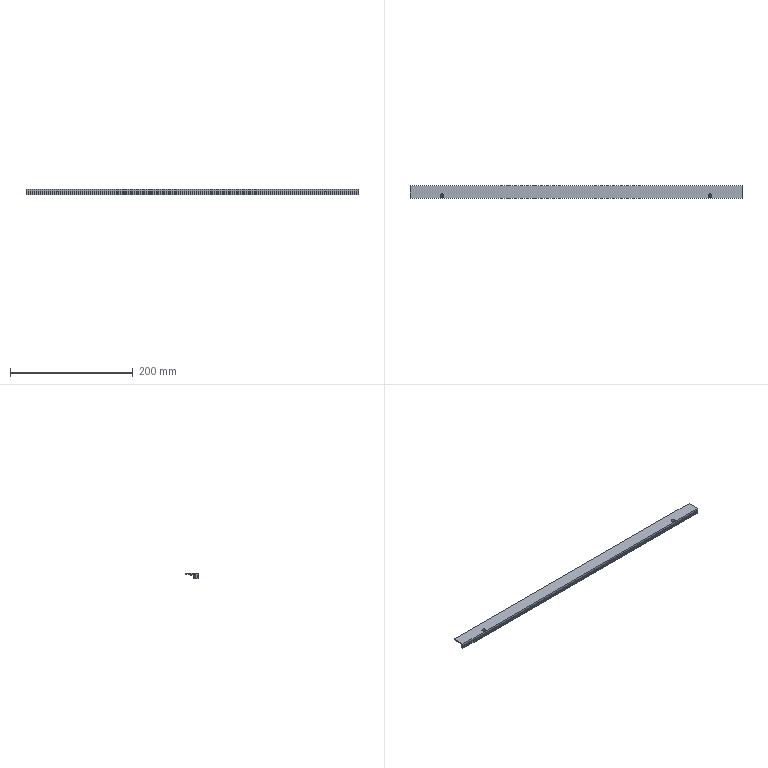Part | SolidWorks | features BaseBody 1 | 1 solid | 40 faces | box 540 x 20 x 9 mm | volume 48974 mm3 | plane 26 | cylinder 12 | cone 2 | commonest cylinder face diameters 6 x6 3.3 x4 2.076 x2
STEP:
#1=CARTESIAN_POINT('',(-215.,-187.,12.));
#2=VERTEX_POINT('',#1);
#3=CARTESIAN_POINT('',(-221.,-187.,12.));
#4=VERTEX_POINT('',#3);
#5=CARTESIAN_POINT('',(-218.,-187.,12.));
#6=DIRECTION('',(0.,0.,-1.));
#7=DIRECTION('',(-1.,0.,0.));
#8=AXIS2_PLACEMENT_3D('',#5,#6,#7);
#9=CIRCLE('',#8,3.);
#10=EDGE_CURVE('',#2,#4,#9,.T.);
#11=ORIENTED_EDGE('',*,*,#10,.F.);
#12=CARTESIAN_POINT('',(-215.,-187.,8.8));
#13=VERTEX_POINT('',#12);
#14=CARTESIAN_POINT('',(-215.,-187.,10.4));
#15=DIRECTION('',(0.,0.,-1.));
#16=VECTOR('',#15,1000.);
#17=LINE('',#14,#16);
#18=EDGE_CURVE('',#2,#13,#17,.T.);
#19=ORIENTED_EDGE('',*,*,#18,.T.);
#20=CARTESIAN_POINT('',(-221.,-187.,8.8));
#21=VERTEX_POINT('',#20);
#22=CARTESIAN_POINT('',(-218.,-187.,8.8));
#23=DIRECTION('',(0.,0.,1.));
#24=DIRECTION('',(-1.,0.,0.));
#25=AXIS2_PLACEMENT_3D('',#22,#23,#24);
#26=CIRCLE('',#25,3.);
#27=EDGE_CURVE('',#21,#13,#26,.T.);
#28=ORIENTED_EDGE('',*,*,#27,.F.);
#29=CARTESIAN_POINT('',(-221.,-187.,10.4));
#30=DIRECTION('',(0.,0.,-1.));
#31=VECTOR('',#30,1000.);
#32=LINE('',#29,#31);
#33=EDGE_CURVE('',#4,#21,#32,.T.);
#34=ORIENTED_EDGE('',*,*,#33,.F.);
#35=EDGE_LOOP('',(#11,#19,#28,#34));
#36=FACE_OUTER_BOUND('',#35,.T.);
#37=CARTESIAN_POINT('',(-218.,-187.,10.4));
#38=DIRECTION('',(0.,0.,-1.));
#39=DIRECTION('',(-1.,0.,0.));
#40=AXIS2_PLACEMENT_3D('',#37,#38,#39);
#41=CYLINDRICAL_SURFACE('',#40,3.);
#42=ADVANCED_FACE('',(#36),#41,.F.);
#43=CARTESIAN_POINT('',(221.,-187.,12.));
#44=VERTEX_POINT('',#43);
#45=CARTESIAN_POINT('',(215.,-187.,12.));
#46=VERTEX_POINT('',#45);
#47=CARTESIAN_POINT('',(218.,-187.,12.));
#48=DIRECTION('',(0.,0.,-1.));
#49=DIRECTION('',(-1.,0.,0.));
#50=AXIS2_PLACEMENT_3D('',#47,#48,#49);
#51=CIRCLE('',#50,3.);
#52=EDGE_CURVE('',#44,#46,#51,.T.);
#53=ORIENTED_EDGE('',*,*,#52,.F.);
#54=CARTESIAN_POINT('',(221.,-187.,8.8));
#55=VERTEX_POINT('',#54);
#56=CARTESIAN_POINT('',(221.,-187.,10.4));
#57=DIRECTION('',(0.,0.,-1.));
#58=VECTOR('',#57,1000.);
#59=LINE('',#56,#58);
#60=EDGE_CURVE('',#44,#55,#59,.T.);
#61=ORIENTED_EDGE('',*,*,#60,.T.);
#62=CARTESIAN_POINT('',(215.,-187.,8.8));
#63=VERTEX_POINT('',#62);
#64=CARTESIAN_POINT('',(218.,-187.,8.8));
#65=DIRECTION('',(0.,0.,1.));
#66=DIRECTION('',(-1.,0.,0.));
#67=AXIS2_PLACEMENT_3D('',#64,#65,#66);
#68=CIRCLE('',#67,3.);
#69=EDGE_CURVE('',#63,#55,#68,.T.);
#70=ORIENTED_EDGE('',*,*,#69,.F.);
#71=CARTESIAN_POINT('',(215.,-187.,10.4));
#72=DIRECTION('',(0.,0.,-1.));
#73=VECTOR('',#72,1000.);
#74=LINE('',#71,#73);
#75=EDGE_CURVE('',#46,#63,#74,.T.);
#76=ORIENTED_EDGE('',*,*,#75,.F.);
#77=EDGE_LOOP('',(#53,#61,#70,#76));
#78=FACE_OUTER_BOUND('',#77,.T.);
#79=CARTESIAN_POINT('',(218.,-187.,10.4));
#80=DIRECTION('',(0.,0.,-1.));
#81=DIRECTION('',(-1.,0.,0.));
#82=AXIS2_PLACEMENT_3D('',#79,#80,#81);
#83=CYLINDRICAL_SURFACE('',#82,3.);
#84=ADVANCED_FACE('',(#78),#83,.F.);
#85=CARTESIAN_POINT('',(-219.65,-187.,8.8));
#86=VERTEX_POINT('',#85);
#87=CARTESIAN_POINT('',(-216.35,-187.,8.8));
#88=VERTEX_POINT('',#87);
#89=CARTESIAN_POINT('',(-218.,-187.,8.8));
#90=DIRECTION('',(0.,0.,1.));
#91=DIRECTION('',(-1.,0.,0.));
#92=AXIS2_PLACEMENT_3D('',#89,#90,#91);
#93=CIRCLE('',#92,1.65);
#94=EDGE_CURVE('',#86,#88,#93,.T.);
#95=ORIENTED_EDGE('',*,*,#94,.T.);
#96=CARTESIAN_POINT('',(-216.35,-187.,3.));
#97=VERTEX_POINT('',#96);
#98=CARTESIAN_POINT('',(-216.35,-187.,7.));
#99=DIRECTION('',(0.,0.,-1.));
#100=VECTOR('',#99,1000.);
#101=LINE('',#98,#100);
#102=EDGE_CURVE('',#88,#97,#101,.T.);
#103=ORIENTED_EDGE('',*,*,#102,.T.);
#104=CARTESIAN_POINT('',(-219.65,-187.,3.));
#105=VERTEX_POINT('',#104);
#106=CARTESIAN_POINT('',(-218.,-187.,3.));
#107=DIRECTION('',(0.,0.,1.));
#108=DIRECTION('',(-1.,0.,0.));
#109=AXIS2_PLACEMENT_3D('',#106,#107,#108);
#110=CIRCLE('',#109,1.65);
#111=EDGE_CURVE('',#105,#97,#110,.T.);
#112=ORIENTED_EDGE('',*,*,#111,.F.);
#113=CARTESIAN_POINT('',(-219.65,-187.,7.));
#114=DIRECTION('',(0.,0.,-1.));
#115=VECTOR('',#114,1000.);
#116=LINE('',#113,#115);
#117=EDGE_CURVE('',#86,#105,#116,.T.);
#118=ORIENTED_EDGE('',*,*,#117,.F.);
#119=EDGE_LOOP('',(#95,#103,#112,#118));
#120=FACE_OUTER_BOUND('',#119,.T.);
#121=CARTESIAN_POINT('',(-218.,-187.,7.));
#122=DIRECTION('',(0.,0.,-1.));
#123=DIRECTION('',(-1.,0.,0.));
#124=AXIS2_PLACEMENT_3D('',#121,#122,#123);
#125=CYLINDRICAL_SURFACE('',#124,1.65);
#126=ADVANCED_FACE('',(#120),#125,.F.);
#127=CARTESIAN_POINT('',(216.35,-187.,8.8));
#128=VERTEX_POINT('',#127);
#129=CARTESIAN_POINT('',(219.65,-187.,8.8));
#130=VERTEX_POINT('',#129);
#131=CARTESIAN_POINT('',(218.,-187.,8.8));
#132=DIRECTION('',(0.,0.,1.));
#133=DIRECTION('',(-1.,0.,0.));
#134=AXIS2_PLACEMENT_3D('',#131,#132,#133);
#135=CIRCLE('',#134,1.65);
#136=EDGE_CURVE('',#128,#130,#135,.T.);
#137=ORIENTED_EDGE('',*,*,#136,.T.);
#138=CARTESIAN_POINT('',(219.65,-187.,3.));
#139=VERTEX_POINT('',#138);
#140=CARTESIAN_POINT('',(219.65,-187.,7.));
#141=DIRECTION('',(0.,0.,-1.));
#142=VECTOR('',#141,1000.);
#143=LINE('',#140,#142);
#144=EDGE_CURVE('',#130,#139,#143,.T.);
#145=ORIENTED_EDGE('',*,*,#144,.T.);
#146=CARTESIAN_POINT('',(216.35,-187.,3.));
#147=VERTEX_POINT('',#146);
#148=CARTESIAN_POINT('',(218.,-187.,3.));
#149=DIRECTION('',(0.,0.,1.));
#150=DIRECTION('',(-1.,0.,0.));
#151=AXIS2_PLACEMENT_3D('',#148,#149,#150);
#152=CIRCLE('',#151,1.65);
#153=EDGE_CURVE('',#147,#139,#152,.T.);
#154=ORIENTED_EDGE('',*,*,#153,.F.);
#155=CARTESIAN_POINT('',(216.35,-187.,7.));
#156=DIRECTION('',(0.,0.,-1.));
#157=VECTOR('',#156,1000.);
#158=LINE('',#155,#157);
#159=EDGE_CURVE('',#128,#147,#158,.T.);
#160=ORIENTED_EDGE('',*,*,#159,.F.);
#161=EDGE_LOOP('',(#137,#145,#154,#160));
#162=FACE_OUTER_BOUND('',#161,.T.);
#163=CARTESIAN_POINT('',(218.,-187.,7.));
#164=DIRECTION('',(0.,0.,-1.));
#165=DIRECTION('',(-1.,0.,0.));
#166=AXIS2_PLACEMENT_3D('',#163,#164,#165);
#167=CYLINDRICAL_SURFACE('',#166,1.65);
#168=ADVANCED_FACE('',(#162),#167,.F.);
#169=CARTESIAN_POINT('',(-254.,-184.,6.223));
#170=VERTEX_POINT('',#169);
#171=CARTESIAN_POINT('',(-254.798,-186.038,6.5));
#172=VERTEX_POINT('',#171);
#173=CARTESIAN_POINT('',(-254.,-184.,6.223));
#174=CARTESIAN_POINT('',(-254.,-184.035,6.096));
#175=CARTESIAN_POINT('',(-254.,-184.093,5.978));
#176=CARTESIAN_POINT('',(-254.009,-184.251,5.77));
#177=CARTESIAN_POINT('',(-254.018,-184.349,5.681));
#178=CARTESIAN_POINT('',(-254.052,-184.569,5.547));
#179=CARTESIAN_POINT('',(-254.078,-184.692,5.501));
#180=CARTESIAN_POINT('',(-254.148,-184.938,5.457));
#181=CARTESIAN_POINT('',(-254.192,-185.064,5.457));
#182=CARTESIAN_POINT('',(-254.343,-185.417,5.52));
#183=CARTESIAN_POINT('',(-254.473,-185.628,5.641));
#184=CARTESIAN_POINT('',(-254.642,-185.858,5.904));
#185=CARTESIAN_POINT('',(-254.696,-185.922,6.008));
#186=CARTESIAN_POINT('',(-254.774,-186.012,6.239));
#187=CARTESIAN_POINT('',(-254.798,-186.038,6.368));
#188=CARTESIAN_POINT('',(-254.798,-186.038,6.5));
#189=B_SPLINE_CURVE_WITH_KNOTS('',3,(#173,#174,#175,#176,#177,#178,#179,#180,#181,#182,#183,#184,#185,#186,#187,#188),.UNSPECIFIED.,.F.,.F.,(4,2,2,2,2,2,2,4),(0.,0.000389,0.000778,0.001167,0.001556,0.002334,0.002723,0.003112),.UNSPECIFIED.);
#190=EDGE_CURVE('',#170,#172,#189,.T.);
#191=ORIENTED_EDGE('',*,*,#190,.T.);
#192=CARTESIAN_POINT('',(-219.34,-186.038,6.5));
#193=VERTEX_POINT('',#192);
#194=CARTESIAN_POINT('',(-150.,-186.038,6.5));
#195=DIRECTION('',(1.,0.,0.));
#196=VECTOR('',#195,1000.);
#197=LINE('',#194,#196);
#198=EDGE_CURVE('',#172,#193,#197,.T.);
#199=ORIENTED_EDGE('',*,*,#198,.T.);
#200=CARTESIAN_POINT('',(-216.66,-186.038,6.5));
#201=VERTEX_POINT('',#200);
#202=CARTESIAN_POINT('',(-219.34,-186.038,6.5));
#203=CARTESIAN_POINT('',(-219.34,-186.038,6.328));
#204=CARTESIAN_POINT('',(-219.31,-185.991,6.154));
#205=CARTESIAN_POINT('',(-219.18,-185.842,5.873));
#206=CARTESIAN_POINT('',(-219.077,-185.741,5.764));
#207=CARTESIAN_POINT('',(-218.821,-185.56,5.619));
#208=CARTESIAN_POINT('',(-218.668,-185.482,5.579));
#209=CARTESIAN_POINT('',(-218.345,-185.378,5.532));
#210=CARTESIAN_POINT('',(-218.172,-185.35,5.523));
#211=CARTESIAN_POINT('',(-217.828,-185.35,5.523));
#212=CARTESIAN_POINT('',(-217.656,-185.377,5.532));
#213=CARTESIAN_POINT('',(-217.413,-185.456,5.567));
#214=CARTESIAN_POINT('',(-217.333,-185.488,5.583));
#215=CARTESIAN_POINT('',(-217.185,-185.563,5.627));
#216=CARTESIAN_POINT('',(-217.115,-185.605,5.655));
#217=CARTESIAN_POINT('',(-216.986,-185.696,5.728));
#218=CARTESIAN_POINT('',(-216.929,-185.743,5.772));
#219=CARTESIAN_POINT('',(-216.83,-185.835,5.88));
#220=CARTESIAN_POINT('',(-216.788,-185.879,5.943));
#221=CARTESIAN_POINT('',(-216.691,-185.991,6.153));
#222=CARTESIAN_POINT('',(-216.66,-186.038,6.326));
#223=CARTESIAN_POINT('',(-216.66,-186.038,6.5));
#224=B_SPLINE_CURVE_WITH_KNOTS('',3,(#202,#203,#204,#205,#206,#207,#208,#209,#210,#211,#212,#213,#214,#215,#216,#217,#218,#219,#220,#221,#222,#223),.UNSPECIFIED.,.F.,.F.,(4,2,2,2,2,2,2,2,2,2,4),(0.004127,0.004642,0.005157,0.005672,0.006187,0.006702,0.00696,0.007217,0.007475,0.007733,0.008248),.UNSPECIFIED.);
#225=EDGE_CURVE('',#193,#201,#224,.T.);
#226=ORIENTED_EDGE('',*,*,#225,.T.);
#227=CARTESIAN_POINT('',(-30.,-186.038,6.5));
#228=VERTEX_POINT('',#227);
#229=CARTESIAN_POINT('',(-150.,-186.038,6.5));
#230=DIRECTION('',(1.,0.,0.));
#231=VECTOR('',#230,1000.);
#232=LINE('',#229,#231);
#233=EDGE_CURVE('',#201,#228,#232,.T.);
#234=ORIENTED_EDGE('',*,*,#233,.T.);
#235=CARTESIAN_POINT('',(-30.,-185.,5.462));
#236=VERTEX_POINT('',#235);
#237=CARTESIAN_POINT('',(-30.,-185.,6.5));
#238=DIRECTION('',(-1.,0.,0.));
#239=DIRECTION('',(0.,1.,0.));
#240=AXIS2_PLACEMENT_3D('',#237,#238,#239);
#241=CIRCLE('',#240,1.038);
#242=EDGE_CURVE('',#236,#228,#241,.T.);
#243=ORIENTED_EDGE('',*,*,#242,.F.);
#244=CARTESIAN_POINT('',(-30.,-183.962,6.5));
#245=VERTEX_POINT('',#244);
#246=CARTESIAN_POINT('',(-30.,-185.,6.5));
#247=DIRECTION('',(-1.,0.,0.));
#248=DIRECTION('',(0.,1.,0.));
#249=AXIS2_PLACEMENT_3D('',#246,#247,#248);
#250=CIRCLE('',#249,1.038);
#251=EDGE_CURVE('',#245,#236,#250,.T.);
#252=ORIENTED_EDGE('',*,*,#251,.F.);
#253=CARTESIAN_POINT('',(-254.,-183.962,6.5));
#254=VERTEX_POINT('',#253);
#255=CARTESIAN_POINT('',(-150.,-183.962,6.5));
#256=DIRECTION('',(1.,0.,0.));
#257=VECTOR('',#256,1000.);
#258=LINE('',#255,#257);
#259=EDGE_CURVE('',#254,#245,#258,.T.);
#260=ORIENTED_EDGE('',*,*,#259,.F.);
#261=CARTESIAN_POINT('',(-254.,-185.,6.5));
#262=DIRECTION('',(-1.,0.,0.));
#263=DIRECTION('',(0.,1.,0.));
#264=AXIS2_PLACEMENT_3D('',#261,#262,#263);
#265=CIRCLE('',#264,1.038);
#266=EDGE_CURVE('',#254,#170,#265,.T.);
#267=ORIENTED_EDGE('',*,*,#266,.T.);
#268=EDGE_LOOP('',(#191,#199,#226,#234,#243,#252,#260,#267));
#269=FACE_OUTER_BOUND('',#268,.T.);
#270=CARTESIAN_POINT('',(-150.,-185.,6.5));
#271=DIRECTION('',(1.,0.,0.));
#272=DIRECTION('',(0.,1.,0.));
#273=AXIS2_PLACEMENT_3D('',#270,#271,#272);
#274=CYLINDRICAL_SURFACE('',#273,1.038);
#275=ADVANCED_FACE('',(#269),#274,.F.);
#276=CARTESIAN_POINT('',(-29.376,-185.,6.5));
#277=VERTEX_POINT('',#276);
#278=CARTESIAN_POINT('',(-30.,-185.,7.538));
#279=VERTEX_POINT('',#278);
#280=CARTESIAN_POINT('',(-30.,-185.,7.538));
#281=DIRECTION('',(-0.515,0.,0.8572));
#282=VECTOR('',#281,1000.);
#283=LINE('',#280,#282);
#284=EDGE_CURVE('',#277,#279,#283,.T.);
#285=ORIENTED_EDGE('',*,*,#284,.F.);
#286=CARTESIAN_POINT('',(-30.,-185.,5.462));
#287=DIRECTION('',(-0.515,0.,-0.8572));
#288=VECTOR('',#287,1000.);
#289=LINE('',#286,#288);
#290=EDGE_CURVE('',#277,#236,#289,.T.);
#291=ORIENTED_EDGE('',*,*,#290,.T.);
#292=ORIENTED_EDGE('',*,*,#242,.T.);
#293=CARTESIAN_POINT('',(-30.,-185.,6.5));
#294=DIRECTION('',(-1.,0.,0.));
#295=DIRECTION('',(0.,1.,0.));
#296=AXIS2_PLACEMENT_3D('',#293,#294,#295);
#297=CIRCLE('',#296,1.038);
#298=EDGE_CURVE('',#228,#279,#297,.T.);
#299=ORIENTED_EDGE('',*,*,#298,.T.);
#300=EDGE_LOOP('',(#285,#291,#292,#299));
#301=FACE_OUTER_BOUND('',#300,.T.);
#302=CARTESIAN_POINT('',(-30.,-185.,6.5));
#303=DIRECTION('',(-1.,0.,0.));
#304=DIRECTION('',(0.,0.,1.));
#305=AXIS2_PLACEMENT_3D('',#302,#303,#304);
#306=CONICAL_SURFACE('',#305,1.038,1.03);
#307=ADVANCED_FACE('',(#301),#306,.F.);
#308=CARTESIAN_POINT('',(-218.,-187.,12.));
#309=DIRECTION('',(0.,0.,-1.));
#310=DIRECTION('',(-1.,0.,0.));
#311=AXIS2_PLACEMENT_3D('',#308,#309,#310);
#312=CIRCLE('',#311,3.);
#313=EDGE_CURVE('',#4,#2,#312,.T.);
#314=ORIENTED_EDGE('',*,*,#313,.T.);
#315=ORIENTED_EDGE('',*,*,#10,.T.);
#316=EDGE_LOOP('',(#314,#315));
#317=FACE_BOUND('',#316,.T.);
#318=CARTESIAN_POINT('',(218.,-187.,12.));
#319=DIRECTION('',(0.,0.,-1.));
#320=DIRECTION('',(-1.,0.,0.));
#321=AXIS2_PLACEMENT_3D('',#318,#319,#320);
#322=CIRCLE('',#321,3.);
#323=EDGE_CURVE('',#46,#44,#322,.T.);
#324=ORIENTED_EDGE('',*,*,#323,.T.);
#325=ORIENTED_EDGE('',*,*,#52,.T.);
#326=EDGE_LOOP('',(#324,#325));
#327=FACE_BOUND('',#326,.T.);
#328=CARTESIAN_POINT('',(-270.,-171.,12.));
#329=VERTEX_POINT('',#328);
#330=CARTESIAN_POINT('',(-270.,-191.,12.));
#331=VERTEX_POINT('',#330);
#332=CARTESIAN_POINT('',(-270.,-171.,12.));
#333=DIRECTION('',(0.,-1.,0.));
#334=VECTOR('',#333,1000.);
#335=LINE('',#332,#334);
#336=EDGE_CURVE('',#329,#331,#335,.T.);
#337=ORIENTED_EDGE('',*,*,#336,.T.);
#338=CARTESIAN_POINT('',(270.,-191.,12.));
#339=VERTEX_POINT('',#338);
#340=CARTESIAN_POINT('',(-270.,-191.,12.));
#341=DIRECTION('',(1.,0.,0.));
#342=VECTOR('',#341,1000.);
#343=LINE('',#340,#342);
#344=EDGE_CURVE('',#331,#339,#343,.T.);
#345=ORIENTED_EDGE('',*,*,#344,.T.);
#346=CARTESIAN_POINT('',(270.,-171.,12.));
#347=VERTEX_POINT('',#346);
#348=CARTESIAN_POINT('',(270.,-171.,12.));
#349=DIRECTION('',(0.,1.,0.));
#350=VECTOR('',#349,1000.);
#351=LINE('',#348,#350);
#352=EDGE_CURVE('',#339,#347,#351,.T.);
#353=ORIENTED_EDGE('',*,*,#352,.T.);
#354=CARTESIAN_POINT('',(-270.,-171.,12.));
#355=DIRECTION('',(-1.,0.,0.));
#356=VECTOR('',#355,1000.);
#357=LINE('',#354,#356);
#358=EDGE_CURVE('',#347,#329,#357,.T.);
#359=ORIENTED_EDGE('',*,*,#358,.T.);
#360=EDGE_LOOP('',(#337,#345,#353,#359));
#361=FACE_OUTER_BOUND('',#360,.T.);
#362=CARTESIAN_POINT('',(-270.,-171.,12.));
#363=DIRECTION('',(0.,0.,1.));
#364=DIRECTION('',(1.,0.,0.));
#365=AXIS2_PLACEMENT_3D('',#362,#363,#364);
#366=PLANE('',#365);
#367=ADVANCED_FACE('',(#317,#327,#361),#366,.T.);
#368=ORIENTED_EDGE('',*,*,#18,.F.);
#369=ORIENTED_EDGE('',*,*,#313,.F.);
#370=ORIENTED_EDGE('',*,*,#33,.T.);
#371=CARTESIAN_POINT('',(-218.,-187.,8.8));
#372=DIRECTION('',(0.,0.,1.));
#373=DIRECTION('',(-1.,0.,0.));
#374=AXIS2_PLACEMENT_3D('',#371,#372,#373);
#375=CIRCLE('',#374,3.);
#376=EDGE_CURVE('',#13,#21,#375,.T.);
#377=ORIENTED_EDGE('',*,*,#376,.F.);
#378=EDGE_LOOP('',(#368,#369,#370,#377));
#379=FACE_OUTER_BOUND('',#378,.T.);
#380=CARTESIAN_POINT('',(-218.,-187.,10.4));
#381=DIRECTION('',(0.,0.,-1.));
#382=DIRECTION('',(-1.,0.,0.));
#383=AXIS2_PLACEMENT_3D('',#380,#381,#382);
#384=CYLINDRICAL_SURFACE('',#383,3.);
#385=ADVANCED_FACE('',(#379),#384,.F.);
#386=ORIENTED_EDGE('',*,*,#60,.F.);
#387=ORIENTED_EDGE('',*,*,#323,.F.);
#388=ORIENTED_EDGE('',*,*,#75,.T.);
#389=CARTESIAN_POINT('',(218.,-187.,8.8));
#390=DIRECTION('',(0.,0.,1.));
#391=DIRECTION('',(-1.,0.,0.));
#392=AXIS2_PLACEMENT_3D('',#389,#390,#391);
#393=CIRCLE('',#392,3.);
#394=EDGE_CURVE('',#55,#63,#393,.T.);
#395=ORIENTED_EDGE('',*,*,#394,.F.);
#396=EDGE_LOOP('',(#386,#387,#388,#395));
#397=FACE_OUTER_BOUND('',#396,.T.);
#398=CARTESIAN_POINT('',(218.,-187.,10.4));
#399=DIRECTION('',(0.,0.,-1.));
#400=DIRECTION('',(-1.,0.,0.));
#401=AXIS2_PLACEMENT_3D('',#398,#399,#400);
#402=CYLINDRICAL_SURFACE('',#401,3.);
#403=ADVANCED_FACE('',(#397),#402,.F.);
#404=ORIENTED_EDGE('',*,*,#344,.F.);
#405=CARTESIAN_POINT('',(-270.,-191.,8.5));
#406=VERTEX_POINT('',#405);
#407=CARTESIAN_POINT('',(-270.,-191.,12.));
#408=DIRECTION('',(0.,0.,-1.));
#409=VECTOR('',#408,1000.);
#410=LINE('',#407,#409);
#411=EDGE_CURVE('',#331,#406,#410,.T.);
#412=ORIENTED_EDGE('',*,*,#411,.T.);
#413=CARTESIAN_POINT('',(270.,-191.,8.5));
#414=VERTEX_POINT('',#413);
#415=CARTESIAN_POINT('',(-270.,-191.,8.5));
#416=DIRECTION('',(1.,0.,0.));
#417=VECTOR('',#416,1000.);
#418=LINE('',#415,#417);
#419=EDGE_CURVE('',#406,#414,#418,.T.);
#420=ORIENTED_EDGE('',*,*,#419,.T.);
#421=CARTESIAN_POINT('',(270.,-191.,12.));
#422=DIRECTION('',(0.,0.,1.));
#423=VECTOR('',#422,1000.);
#424=LINE('',#421,#423);
#425=EDGE_CURVE('',#414,#339,#424,.T.);
#426=ORIENTED_EDGE('',*,*,#425,.T.);
#427=EDGE_LOOP('',(#404,#412,#420,#426));
#428=FACE_OUTER_BOUND('',#427,.T.);
#429=CARTESIAN_POINT('',(-270.,-191.,12.));
#430=DIRECTION('',(0.,-1.,0.));
#431=DIRECTION('',(0.,0.,-1.));
#432=AXIS2_PLACEMENT_3D('',#429,#430,#431);
#433=PLANE('',#432);
#434=ADVANCED_FACE('',(#428),#433,.T.);
#435=CARTESIAN_POINT('',(-270.,-187.,3.));
#436=VERTEX_POINT('',#435);
#437=CARTESIAN_POINT('',(-270.,-191.,3.));
#438=VERTEX_POINT('',#437);
#439=CARTESIAN_POINT('',(-270.,-181.,3.));
#440=DIRECTION('',(0.,-1.,0.));
#441=VECTOR('',#440,1000.);
#442=LINE('',#439,#441);
#443=EDGE_CURVE('',#436,#438,#442,.T.);
#444=ORIENTED_EDGE('',*,*,#443,.T.);
#445=CARTESIAN_POINT('',(-270.,-191.,4.5));
#446=VERTEX_POINT('',#445);
#447=CARTESIAN_POINT('',(-270.,-191.,12.));
#448=DIRECTION('',(0.,0.,-1.));
#449=VECTOR('',#448,1000.);
#450=LINE('',#447,#449);
#451=EDGE_CURVE('',#446,#438,#450,.T.);
#452=ORIENTED_EDGE('',*,*,#451,.F.);
#453=CARTESIAN_POINT('',(-270.,-190.,4.5));
#454=VERTEX_POINT('',#453);
#455=CARTESIAN_POINT('',(-270.,-191.,4.5));
#456=DIRECTION('',(0.,1.,0.));
#457=VECTOR('',#456,1000.);
#458=LINE('',#455,#457);
#459=EDGE_CURVE('',#446,#454,#458,.T.);
#460=ORIENTED_EDGE('',*,*,#459,.T.);
#461=CARTESIAN_POINT('',(-270.,-190.,6.));
#462=VERTEX_POINT('',#461);
#463=CARTESIAN_POINT('',(-270.,-190.,4.5));
#464=DIRECTION('',(0.,0.,1.));
#465=VECTOR('',#464,1000.);
#466=LINE('',#463,#465);
#467=EDGE_CURVE('',#454,#462,#466,.T.);
#468=ORIENTED_EDGE('',*,*,#467,.T.);
#469=CARTESIAN_POINT('',(-270.,-191.,6.));
#470=VERTEX_POINT('',#469);
#471=CARTESIAN_POINT('',(-270.,-190.,6.));
#472=DIRECTION('',(0.,-1.,0.));
#473=VECTOR('',#472,1000.);
#474=LINE('',#471,#473);
#475=EDGE_CURVE('',#462,#470,#474,.T.);
#476=ORIENTED_EDGE('',*,*,#475,.T.);
#477=CARTESIAN_POINT('',(-270.,-191.,7.));
#478=VERTEX_POINT('',#477);
#479=CARTESIAN_POINT('',(-270.,-191.,12.));
#480=DIRECTION('',(0.,0.,-1.));
#481=VECTOR('',#480,1000.);
#482=LINE('',#479,#481);
#483=EDGE_CURVE('',#478,#470,#482,.T.);
#484=ORIENTED_EDGE('',*,*,#483,.F.);
#485=CARTESIAN_POINT('',(-270.,-190.,7.));
#486=VERTEX_POINT('',#485);
#487=CARTESIAN_POINT('',(-270.,-191.,7.));
#488=DIRECTION('',(0.,1.,0.));
#489=VECTOR('',#488,1000.);
#490=LINE('',#487,#489);
#491=EDGE_CURVE('',#478,#486,#490,.T.);
#492=ORIENTED_EDGE('',*,*,#491,.T.);
#493=CARTESIAN_POINT('',(-270.,-190.,8.5));
#494=VERTEX_POINT('',#493);
#495=CARTESIAN_POINT('',(-270.,-190.,7.));
#496=DIRECTION('',(0.,0.,1.));
#497=VECTOR('',#496,1000.);
#498=LINE('',#495,#497);
#499=EDGE_CURVE('',#486,#494,#498,.T.);
#500=ORIENTED_EDGE('',*,*,#499,.T.);
#501=CARTESIAN_POINT('',(-270.,-181.,8.5));
#502=DIRECTION('',(0.,-1.,0.));
#503=VECTOR('',#502,1000.);
#504=LINE('',#501,#503);
#505=EDGE_CURVE('',#494,#406,#504,.T.);
#506=ORIENTED_EDGE('',*,*,#505,.T.);
#507=ORIENTED_EDGE('',*,*,#411,.F.);
#508=ORIENTED_EDGE('',*,*,#336,.F.);
#509=CARTESIAN_POINT('',(-270.,-171.,10.5));
#510=VERTEX_POINT('',#509);
#511=CARTESIAN_POINT('',(-270.,-171.,7.5));
#512=DIRECTION('',(0.,0.,-1.));
#513=VECTOR('',#512,1000.);
#514=LINE('',#511,#513);
#515=EDGE_CURVE('',#329,#510,#514,.T.);
#516=ORIENTED_EDGE('',*,*,#515,.T.);
#517=CARTESIAN_POINT('',(-270.,-187.,10.5));
#518=VERTEX_POINT('',#517);
#519=CARTESIAN_POINT('',(-270.,-181.,10.5));
#520=DIRECTION('',(0.,-1.,0.));
#521=VECTOR('',#520,1000.);
#522=LINE('',#519,#521);
#523=EDGE_CURVE('',#510,#518,#522,.T.);
#524=ORIENTED_EDGE('',*,*,#523,.T.);
#525=CARTESIAN_POINT('',(-270.,-187.,7.5));
#526=DIRECTION('',(0.,0.,-1.));
#527=VECTOR('',#526,1000.);
#528=LINE('',#525,#527);
#529=EDGE_CURVE('',#518,#436,#528,.T.);
#530=ORIENTED_EDGE('',*,*,#529,.T.);
#531=EDGE_LOOP('',(#444,#452,#460,#468,#476,#484,#492,#500,#506,#507,#508,#516,#524,#530));
#532=FACE_OUTER_BOUND('',#531,.T.);
#533=CARTESIAN_POINT('',(-270.,-181.,7.5));
#534=DIRECTION('',(-1.,0.,0.));
#535=DIRECTION('',(0.,-1.,0.));
#536=AXIS2_PLACEMENT_3D('',#533,#534,#535);
#537=PLANE('',#536);
#538=ADVANCED_FACE('',(#532),#537,.T.);
#539=ORIENTED_EDGE('',*,*,#515,.F.);
#540=ORIENTED_EDGE('',*,*,#358,.F.);
#541=CARTESIAN_POINT('',(270.,-171.,10.5));
#542=VERTEX_POINT('',#541);
#543=CARTESIAN_POINT('',(270.,-171.,10.5));
#544=DIRECTION('',(0.,0.,-1.));
#545=VECTOR('',#544,1000.);
#546=LINE('',#543,#545);
#547=EDGE_CURVE('',#347,#542,#546,.T.);
#548=ORIENTED_EDGE('',*,*,#547,.T.);
#549=CARTESIAN_POINT('',(-270.,-171.,10.5));
#550=DIRECTION('',(-1.,0.,0.));
#551=VECTOR('',#550,1000.);
#552=LINE('',#549,#551);
#553=EDGE_CURVE('',#542,#510,#552,.T.);
#554=ORIENTED_EDGE('',*,*,#553,.T.);
#555=EDGE_LOOP('',(#539,#540,#548,#554));
#556=FACE_OUTER_BOUND('',#555,.T.);
#557=CARTESIAN_POINT('',(-270.,-171.,10.5));
#558=DIRECTION('',(0.,1.,0.));
#559=DIRECTION('',(0.,0.,1.));
#560=AXIS2_PLACEMENT_3D('',#557,#558,#559);
#561=PLANE('',#560);
#562=ADVANCED_FACE('',(#556),#561,.T.);
#563=CARTESIAN_POINT('',(270.,-191.,6.));
#564=VERTEX_POINT('',#563);
#565=CARTESIAN_POINT('',(270.,-190.,6.));
#566=VERTEX_POINT('',#565);
#567=CARTESIAN_POINT('',(270.,-190.,6.));
#568=DIRECTION('',(0.,1.,0.));
#569=VECTOR('',#568,1000.);
#570=LINE('',#567,#569);
#571=EDGE_CURVE('',#564,#566,#570,.T.);
#572=ORIENTED_EDGE('',*,*,#571,.T.);
#573=CARTESIAN_POINT('',(270.,-190.,4.5));
#574=VERTEX_POINT('',#573);
#575=CARTESIAN_POINT('',(270.,-190.,4.5));
#576=DIRECTION('',(0.,0.,-1.));
#577=VECTOR('',#576,1000.);
#578=LINE('',#575,#577);
#579=EDGE_CURVE('',#566,#574,#578,.T.);
#580=ORIENTED_EDGE('',*,*,#579,.T.);
#581=CARTESIAN_POINT('',(270.,-191.,4.5));
#582=VERTEX_POINT('',#581);
#583=CARTESIAN_POINT('',(270.,-191.,4.5));
#584=DIRECTION('',(0.,-1.,0.));
#585=VECTOR('',#584,1000.);
#586=LINE('',#583,#585);
#587=EDGE_CURVE('',#574,#582,#586,.T.);
#588=ORIENTED_EDGE('',*,*,#587,.T.);
#589=CARTESIAN_POINT('',(270.,-191.,3.));
#590=VERTEX_POINT('',#589);
#591=CARTESIAN_POINT('',(270.,-191.,12.));
#592=DIRECTION('',(0.,0.,1.));
#593=VECTOR('',#592,1000.);
#594=LINE('',#591,#593);
#595=EDGE_CURVE('',#590,#582,#594,.T.);
#596=ORIENTED_EDGE('',*,*,#595,.F.);
#597=CARTESIAN_POINT('',(270.,-187.,3.));
#598=VERTEX_POINT('',#597);
#599=CARTESIAN_POINT('',(270.,-181.,3.));
#600=DIRECTION('',(0.,1.,0.));
#601=VECTOR('',#600,1000.);
#602=LINE('',#599,#601);
#603=EDGE_CURVE('',#590,#598,#602,.T.);
#604=ORIENTED_EDGE('',*,*,#603,.T.);
#605=CARTESIAN_POINT('',(270.,-187.,10.5));
#606=VERTEX_POINT('',#605);
#607=CARTESIAN_POINT('',(270.,-187.,7.5));
#608=DIRECTION('',(0.,0.,1.));
#609=VECTOR('',#608,1000.);
#610=LINE('',#607,#609);
#611=EDGE_CURVE('',#598,#606,#610,.T.);
#612=ORIENTED_EDGE('',*,*,#611,.T.);
#613=CARTESIAN_POINT('',(270.,-181.,10.5));
#614=DIRECTION('',(0.,1.,0.));
#615=VECTOR('',#614,1000.);
#616=LINE('',#613,#615);
#617=EDGE_CURVE('',#606,#542,#616,.T.);
#618=ORIENTED_EDGE('',*,*,#617,.T.);
#619=ORIENTED_EDGE('',*,*,#547,.F.);
#620=ORIENTED_EDGE('',*,*,#352,.F.);
#621=ORIENTED_EDGE('',*,*,#425,.F.);
#622=CARTESIAN_POINT('',(270.,-190.,8.5));
#623=VERTEX_POINT('',#622);
#624=CARTESIAN_POINT('',(270.,-181.,8.5));
#625=DIRECTION('',(0.,1.,0.));
#626=VECTOR('',#625,1000.);
#627=LINE('',#624,#626);
#628=EDGE_CURVE('',#414,#623,#627,.T.);
#629=ORIENTED_EDGE('',*,*,#628,.T.);
#630=CARTESIAN_POINT('',(270.,-190.,7.));
#631=VERTEX_POINT('',#630);
#632=CARTESIAN_POINT('',(270.,-190.,7.));
#633=DIRECTION('',(0.,0.,-1.));
#634=VECTOR('',#633,1000.);
#635=LINE('',#632,#634);
#636=EDGE_CURVE('',#623,#631,#635,.T.);
#637=ORIENTED_EDGE('',*,*,#636,.T.);
#638=CARTESIAN_POINT('',(270.,-191.,7.));
#639=VERTEX_POINT('',#638);
#640=CARTESIAN_POINT('',(270.,-191.,7.));
#641=DIRECTION('',(0.,-1.,0.));
#642=VECTOR('',#641,1000.);
#643=LINE('',#640,#642);
#644=EDGE_CURVE('',#631,#639,#643,.T.);
#645=ORIENTED_EDGE('',*,*,#644,.T.);
#646=CARTESIAN_POINT('',(270.,-191.,12.));
#647=DIRECTION('',(0.,0.,1.));
#648=VECTOR('',#647,1000.);
#649=LINE('',#646,#648);
#650=EDGE_CURVE('',#564,#639,#649,.T.);
#651=ORIENTED_EDGE('',*,*,#650,.F.);
#652=EDGE_LOOP('',(#572,#580,#588,#596,#604,#612,#618,#619,#620,#621,#629,#637,#645,#651));
#653=FACE_OUTER_BOUND('',#652,.T.);
#654=CARTESIAN_POINT('',(270.,-181.,7.5));
#655=DIRECTION('',(1.,0.,0.));
#656=DIRECTION('',(0.,1.,0.));
#657=AXIS2_PLACEMENT_3D('',#654,#655,#656);
#658=PLANE('',#657);
#659=ADVANCED_FACE('',(#653),#658,.T.);
#660=ORIENTED_EDGE('',*,*,#94,.F.);
#661=CARTESIAN_POINT('',(-218.,-187.,8.8));
#662=DIRECTION('',(0.,0.,1.));
#663=DIRECTION('',(-1.,0.,0.));
#664=AXIS2_PLACEMENT_3D('',#661,#662,#663);
#665=CIRCLE('',#664,1.65);
#666=EDGE_CURVE('',#88,#86,#665,.T.);
#667=ORIENTED_EDGE('',*,*,#666,.F.);
#668=EDGE_LOOP('',(#660,#667));
#669=FACE_BOUND('',#668,.T.);
#670=ORIENTED_EDGE('',*,*,#27,.T.);
#671=ORIENTED_EDGE('',*,*,#376,.T.);
#672=EDGE_LOOP('',(#670,#671));
#673=FACE_OUTER_BOUND('',#672,.T.);
#674=CARTESIAN_POINT('',(-218.,-187.,8.8));
#675=DIRECTION('',(0.,0.,-1.));
#676=DIRECTION('',(-1.,0.,0.));
#677=AXIS2_PLACEMENT_3D('',#674,#675,#676);
#678=PLANE('',#677);
#679=ADVANCED_FACE('',(#669,#673),#678,.F.);
#680=ORIENTED_EDGE('',*,*,#136,.F.);
#681=CARTESIAN_POINT('',(218.,-187.,8.8));
#682=DIRECTION('',(0.,0.,1.));
#683=DIRECTION('',(-1.,0.,0.));
#684=AXIS2_PLACEMENT_3D('',#681,#682,#683);
#685=CIRCLE('',#684,1.65);
#686=EDGE_CURVE('',#130,#128,#685,.T.);
#687=ORIENTED_EDGE('',*,*,#686,.F.);
#688=EDGE_LOOP('',(#680,#687));
#689=FACE_BOUND('',#688,.T.);
#690=ORIENTED_EDGE('',*,*,#69,.T.);
#691=ORIENTED_EDGE('',*,*,#394,.T.);
#692=EDGE_LOOP('',(#690,#691));
#693=FACE_OUTER_BOUND('',#692,.T.);
#694=CARTESIAN_POINT('',(218.,-187.,8.8));
#695=DIRECTION('',(0.,0.,-1.));
#696=DIRECTION('',(-1.,0.,0.));
#697=AXIS2_PLACEMENT_3D('',#694,#695,#696);
#698=PLANE('',#697);
#699=ADVANCED_FACE('',(#689,#693),#698,.F.);
#700=ORIENTED_EDGE('',*,*,#419,.F.);
#701=ORIENTED_EDGE('',*,*,#505,.F.);
#702=CARTESIAN_POINT('',(-270.,-190.,8.5));
#703=DIRECTION('',(-1.,0.,0.));
#704=VECTOR('',#703,1000.);
#705=LINE('',#702,#704);
#706=EDGE_CURVE('',#623,#494,#705,.T.);
#707=ORIENTED_EDGE('',*,*,#706,.F.);
#708=ORIENTED_EDGE('',*,*,#628,.F.);
#709=EDGE_LOOP('',(#700,#701,#707,#708));
#710=FACE_OUTER_BOUND('',#709,.T.);
#711=CARTESIAN_POINT('',(-270.,-190.,8.5));
#712=DIRECTION('',(0.,0.,1.));
#713=DIRECTION('',(1.,0.,0.));
#714=AXIS2_PLACEMENT_3D('',#711,#712,#713);
#715=PLANE('',#714);
#716=ADVANCED_FACE('',(#710),#715,.F.);
#717=ORIENTED_EDGE('',*,*,#111,.T.);
#718=CARTESIAN_POINT('',(-218.,-187.,3.));
#719=DIRECTION('',(0.,0.,1.));
#720=DIRECTION('',(-1.,0.,0.));
#721=AXIS2_PLACEMENT_3D('',#718,#719,#720);
#722=CIRCLE('',#721,1.65);
#723=EDGE_CURVE('',#97,#105,#722,.T.);
#724=ORIENTED_EDGE('',*,*,#723,.T.);
#725=EDGE_LOOP('',(#717,#724));
#726=FACE_BOUND('',#725,.T.);
#727=ORIENTED_EDGE('',*,*,#153,.T.);
#728=CARTESIAN_POINT('',(218.,-187.,3.));
#729=DIRECTION('',(0.,0.,1.));
#730=DIRECTION('',(-1.,0.,0.));
#731=AXIS2_PLACEMENT_3D('',#728,#729,#730);
#732=CIRCLE('',#731,1.65);
#733=EDGE_CURVE('',#139,#147,#732,.T.);
#734=ORIENTED_EDGE('',*,*,#733,.T.);
#735=EDGE_LOOP('',(#727,#734));
#736=FACE_BOUND('',#735,.T.);
#737=CARTESIAN_POINT('',(-254.,-184.,3.));
#738=VERTEX_POINT('',#737);
#739=CARTESIAN_POINT('',(-254.,-183.,3.));
#740=VERTEX_POINT('',#739);
#741=CARTESIAN_POINT('',(-254.,-184.,3.));
#742=DIRECTION('',(0.,1.,0.));
#743=VECTOR('',#742,1000.);
#744=LINE('',#741,#743);
#745=EDGE_CURVE('',#738,#740,#744,.T.);
#746=ORIENTED_EDGE('',*,*,#745,.T.);
#747=CARTESIAN_POINT('',(254.,-183.,3.));
#748=VERTEX_POINT('',#747);
#749=CARTESIAN_POINT('',(-270.,-183.,3.));
#750=DIRECTION('',(1.,0.,0.));
#751=VECTOR('',#750,1000.);
#752=LINE('',#749,#751);
#753=EDGE_CURVE('',#740,#748,#752,.T.);
#754=ORIENTED_EDGE('',*,*,#753,.T.);
#755=CARTESIAN_POINT('',(254.,-184.,3.));
#756=VERTEX_POINT('',#755);
#757=CARTESIAN_POINT('',(254.,-171.,3.));
#758=DIRECTION('',(0.,-1.,0.));
#759=VECTOR('',#758,1000.);
#760=LINE('',#757,#759);
#761=EDGE_CURVE('',#748,#756,#760,.T.);
#762=ORIENTED_EDGE('',*,*,#761,.T.);
#763=CARTESIAN_POINT('',(257.,-187.,3.));
#764=VERTEX_POINT('',#763);
#765=CARTESIAN_POINT('',(257.,-184.,3.));
#766=DIRECTION('',(0.,0.,1.));
#767=DIRECTION('',(1.,0.,0.));
#768=AXIS2_PLACEMENT_3D('',#765,#766,#767);
#769=CIRCLE('',#768,3.);
#770=EDGE_CURVE('',#756,#764,#769,.T.);
#771=ORIENTED_EDGE('',*,*,#770,.T.);
#772=CARTESIAN_POINT('',(-270.,-187.,3.));
#773=DIRECTION('',(1.,0.,0.));
#774=VECTOR('',#773,1000.);
#775=LINE('',#772,#774);
#776=EDGE_CURVE('',#764,#598,#775,.T.);
#777=ORIENTED_EDGE('',*,*,#776,.T.);
#778=ORIENTED_EDGE('',*,*,#603,.F.);
#779=CARTESIAN_POINT('',(-270.,-191.,3.));
#780=DIRECTION('',(-1.,0.,0.));
#781=VECTOR('',#780,1000.);
#782=LINE('',#779,#781);
#783=EDGE_CURVE('',#590,#438,#782,.T.);
#784=ORIENTED_EDGE('',*,*,#783,.T.);
#785=ORIENTED_EDGE('',*,*,#443,.F.);
#786=CARTESIAN_POINT('',(-257.,-187.,3.));
#787=VERTEX_POINT('',#786);
#788=CARTESIAN_POINT('',(-270.,-187.,3.));
#789=DIRECTION('',(1.,0.,0.));
#790=VECTOR('',#789,1000.);
#791=LINE('',#788,#790);
#792=EDGE_CURVE('',#436,#787,#791,.T.);
#793=ORIENTED_EDGE('',*,*,#792,.T.);
#794=CARTESIAN_POINT('',(-257.,-184.,3.));
#795=DIRECTION('',(0.,0.,1.));
#796=DIRECTION('',(1.,0.,0.));
#797=AXIS2_PLACEMENT_3D('',#794,#795,#796);
#798=CIRCLE('',#797,3.);
#799=EDGE_CURVE('',#787,#738,#798,.T.);
#800=ORIENTED_EDGE('',*,*,#799,.T.);
#801=EDGE_LOOP('',(#746,#754,#762,#771,#777,#778,#784,#785,#793,#800));
#802=FACE_OUTER_BOUND('',#801,.T.);
#803=CARTESIAN_POINT('',(-270.,-191.,3.));
#804=DIRECTION('',(0.,0.,-1.));
#805=DIRECTION('',(-1.,0.,0.));
#806=AXIS2_PLACEMENT_3D('',#803,#804,#805);
#807=PLANE('',#806);
#808=ADVANCED_FACE('',(#726,#736,#802),#807,.T.);
#809=ORIENTED_EDGE('',*,*,#529,.F.);
#810=CARTESIAN_POINT('',(-257.,-187.,10.5));
#811=VERTEX_POINT('',#810);
#812=CARTESIAN_POINT('',(-270.,-187.,10.5));
#813=DIRECTION('',(-1.,0.,0.));
#814=VECTOR('',#813,1000.);
#815=LINE('',#812,#814);
#816=EDGE_CURVE('',#811,#518,#815,.T.);
#817=ORIENTED_EDGE('',*,*,#816,.F.);
#818=CARTESIAN_POINT('',(-257.,-187.,3.));
#819=DIRECTION('',(0.,0.,1.));
#820=VECTOR('',#819,1000.);
#821=LINE('',#818,#820);
#822=EDGE_CURVE('',#787,#811,#821,.T.);
#823=ORIENTED_EDGE('',*,*,#822,.F.);
#824=ORIENTED_EDGE('',*,*,#792,.F.);
#825=EDGE_LOOP('',(#809,#817,#823,#824));
#826=FACE_OUTER_BOUND('',#825,.T.);
#827=CARTESIAN_POINT('',(-270.,-187.,3.));
#828=DIRECTION('',(0.,-1.,0.));
#829=DIRECTION('',(0.,0.,-1.));
#830=AXIS2_PLACEMENT_3D('',#827,#828,#829);
#831=PLANE('',#830);
#832=ADVANCED_FACE('',(#826),#831,.F.);
#833=CARTESIAN_POINT('',(257.,-187.,10.5));
#834=VERTEX_POINT('',#833);
#835=CARTESIAN_POINT('',(254.,-184.,10.5));
#836=VERTEX_POINT('',#835);
#837=CARTESIAN_POINT('',(257.,-184.,10.5));
#838=DIRECTION('',(0.,0.,-1.));
#839=DIRECTION('',(1.,0.,0.));
#840=AXIS2_PLACEMENT_3D('',#837,#838,#839);
#841=CIRCLE('',#840,3.);
#842=EDGE_CURVE('',#834,#836,#841,.T.);
#843=ORIENTED_EDGE('',*,*,#842,.T.);
#844=CARTESIAN_POINT('',(254.,-178.3,10.5));
#845=VERTEX_POINT('',#844);
#846=CARTESIAN_POINT('',(254.,-178.3,10.5));
#847=DIRECTION('',(0.,1.,0.));
#848=VECTOR('',#847,1000.);
#849=LINE('',#846,#848);
#850=EDGE_CURVE('',#836,#845,#849,.T.);
#851=ORIENTED_EDGE('',*,*,#850,.T.);
#852=CARTESIAN_POINT('',(-254.,-178.3,10.5));
#853=VERTEX_POINT('',#852);
#854=CARTESIAN_POINT('',(-270.,-178.3,10.5));
#855=DIRECTION('',(-1.,0.,0.));
#856=VECTOR('',#855,1000.);
#857=LINE('',#854,#856);
#858=EDGE_CURVE('',#845,#853,#857,.T.);
#859=ORIENTED_EDGE('',*,*,#858,.T.);
#860=CARTESIAN_POINT('',(-254.,-184.,10.5));
#861=VERTEX_POINT('',#860);
#862=CARTESIAN_POINT('',(-254.,-178.3,10.5));
#863=DIRECTION('',(0.,-1.,0.));
#864=VECTOR('',#863,1000.);
#865=LINE('',#862,#864);
#866=EDGE_CURVE('',#853,#861,#865,.T.);
#867=ORIENTED_EDGE('',*,*,#866,.T.);
#868=CARTESIAN_POINT('',(-257.,-184.,10.5));
#869=DIRECTION('',(0.,0.,-1.));
#870=DIRECTION('',(1.,0.,0.));
#871=AXIS2_PLACEMENT_3D('',#868,#869,#870);
#872=CIRCLE('',#871,3.);
#873=EDGE_CURVE('',#861,#811,#872,.T.);
#874=ORIENTED_EDGE('',*,*,#873,.T.);
#875=ORIENTED_EDGE('',*,*,#816,.T.);
#876=ORIENTED_EDGE('',*,*,#523,.F.);
#877=ORIENTED_EDGE('',*,*,#553,.F.);
#878=ORIENTED_EDGE('',*,*,#617,.F.);
#879=CARTESIAN_POINT('',(-270.,-187.,10.5));
#880=DIRECTION('',(-1.,0.,0.));
#881=VECTOR('',#880,1000.);
#882=LINE('',#879,#881);
#883=EDGE_CURVE('',#606,#834,#882,.T.);
#884=ORIENTED_EDGE('',*,*,#883,.T.);
#885=EDGE_LOOP('',(#843,#851,#859,#867,#874,#875,#876,#877,#878,#884));
#886=FACE_OUTER_BOUND('',#885,.T.);
#887=CARTESIAN_POINT('',(-270.,-178.3,10.5));
#888=DIRECTION('',(0.,0.,-1.));
#889=DIRECTION('',(0.,1.,0.));
#890=AXIS2_PLACEMENT_3D('',#887,#888,#889);
#891=PLANE('',#890);
#892=ADVANCED_FACE('',(#886),#891,.T.);
#893=CARTESIAN_POINT('',(257.,-187.,3.));
#894=DIRECTION('',(0.,0.,-1.));
#895=VECTOR('',#894,1000.);
#896=LINE('',#893,#895);
#897=EDGE_CURVE('',#834,#764,#896,.T.);
#898=ORIENTED_EDGE('',*,*,#897,.F.);
#899=ORIENTED_EDGE('',*,*,#883,.F.);
#900=ORIENTED_EDGE('',*,*,#611,.F.);
#901=ORIENTED_EDGE('',*,*,#776,.F.);
#902=EDGE_LOOP('',(#898,#899,#900,#901));
#903=FACE_OUTER_BOUND('',#902,.T.);
#904=CARTESIAN_POINT('',(257.,-187.,3.));
#905=DIRECTION('',(0.,-1.,0.));
#906=DIRECTION('',(0.,0.,-1.));
#907=AXIS2_PLACEMENT_3D('',#904,#905,#906);
#908=PLANE('',#907);
#909=ADVANCED_FACE('',(#903),#908,.F.);
#910=ORIENTED_EDGE('',*,*,#102,.F.);
#911=ORIENTED_EDGE('',*,*,#666,.T.);
#912=ORIENTED_EDGE('',*,*,#117,.T.);
#913=ORIENTED_EDGE('',*,*,#723,.F.);
#914=EDGE_LOOP('',(#910,#911,#912,#913));
#915=FACE_OUTER_BOUND('',#914,.T.);
#916=CARTESIAN_POINT('',(-216.66,-186.038,6.5));
#917=CARTESIAN_POINT('',(-216.66,-186.038,6.674));
#918=CARTESIAN_POINT('',(-216.69,-185.992,6.845));
#919=CARTESIAN_POINT('',(-216.821,-185.842,7.128));
#920=CARTESIAN_POINT('',(-216.923,-185.74,7.236));
#921=CARTESIAN_POINT('',(-217.115,-185.605,7.345));
#922=CARTESIAN_POINT('',(-217.186,-185.563,7.373));
#923=CARTESIAN_POINT('',(-217.334,-185.488,7.417));
#924=CARTESIAN_POINT('',(-217.412,-185.456,7.433));
#925=CARTESIAN_POINT('',(-217.657,-185.377,7.469));
#926=CARTESIAN_POINT('',(-217.829,-185.35,7.477));
#927=CARTESIAN_POINT('',(-218.174,-185.35,7.477));
#928=CARTESIAN_POINT('',(-218.345,-185.377,7.468));
#929=CARTESIAN_POINT('',(-218.589,-185.456,7.432));
#930=CARTESIAN_POINT('',(-218.667,-185.489,7.417));
#931=CARTESIAN_POINT('',(-218.816,-185.563,7.373));
#932=CARTESIAN_POINT('',(-218.887,-185.606,7.344));
#933=CARTESIAN_POINT('',(-219.014,-185.696,7.272));
#934=CARTESIAN_POINT('',(-219.072,-185.744,7.227));
#935=CARTESIAN_POINT('',(-219.171,-185.836,7.119));
#936=CARTESIAN_POINT('',(-219.212,-185.879,7.057));
#937=CARTESIAN_POINT('',(-219.31,-185.992,6.845));
#938=CARTESIAN_POINT('',(-219.34,-186.038,6.672));
#939=CARTESIAN_POINT('',(-219.34,-186.038,6.5));
#940=B_SPLINE_CURVE_WITH_KNOTS('',3,(#916,#917,#918,#919,#920,#921,#922,#923,#924,#925,#926,#927,#928,#929,#930,#931,#932,#933,#934,#935,#936,#937,#938,#939),.UNSPECIFIED.,.F.,.F.,(4,2,2,2,2,2,2,2,2,2,2,4),(0.,0.0005158,0.001032,0.00129,0.001548,0.002063,0.002579,0.002837,0.003095,0.003353,0.003611,0.004127),.UNSPECIFIED.);
#941=EDGE_CURVE('',#201,#193,#940,.T.);
#942=ORIENTED_EDGE('',*,*,#941,.F.);
#943=ORIENTED_EDGE('',*,*,#225,.F.);
#944=EDGE_LOOP('',(#942,#943));
#945=FACE_BOUND('',#944,.T.);
#946=CARTESIAN_POINT('',(-218.,-187.,7.));
#947=DIRECTION('',(0.,0.,-1.));
#948=DIRECTION('',(-1.,0.,0.));
#949=AXIS2_PLACEMENT_3D('',#946,#947,#948);
#950=CYLINDRICAL_SURFACE('',#949,1.65);
#951=ADVANCED_FACE('',(#915,#945),#950,.F.);
#952=ORIENTED_EDGE('',*,*,#144,.F.);
#953=ORIENTED_EDGE('',*,*,#686,.T.);
#954=ORIENTED_EDGE('',*,*,#159,.T.);
#955=ORIENTED_EDGE('',*,*,#733,.F.);
#956=EDGE_LOOP('',(#952,#953,#954,#955));
#957=FACE_OUTER_BOUND('',#956,.T.);
#958=CARTESIAN_POINT('',(218.,-187.,7.));
#959=DIRECTION('',(0.,0.,-1.));
#960=DIRECTION('',(-1.,0.,0.));
#961=AXIS2_PLACEMENT_3D('',#958,#959,#960);
#962=CYLINDRICAL_SURFACE('',#961,1.65);
#963=ADVANCED_FACE('',(#957),#962,.F.);
#964=ORIENTED_EDGE('',*,*,#706,.T.);
#965=ORIENTED_EDGE('',*,*,#499,.F.);
#966=CARTESIAN_POINT('',(-270.,-190.,7.));
#967=DIRECTION('',(-1.,0.,0.));
#968=VECTOR('',#967,1000.);
#969=LINE('',#966,#968);
#970=EDGE_CURVE('',#631,#486,#969,.T.);
#971=ORIENTED_EDGE('',*,*,#970,.F.);
#972=ORIENTED_EDGE('',*,*,#636,.F.);
#973=EDGE_LOOP('',(#964,#965,#971,#972));
#974=FACE_OUTER_BOUND('',#973,.T.);
#975=CARTESIAN_POINT('',(-270.,-190.,7.));
#976=DIRECTION('',(0.,1.,0.));
#977=DIRECTION('',(-1.,0.,0.));
#978=AXIS2_PLACEMENT_3D('',#975,#976,#977);
#979=PLANE('',#978);
#980=ADVANCED_FACE('',(#974),#979,.F.);
#981=CARTESIAN_POINT('',(-254.,-183.,9.));
#982=VERTEX_POINT('',#981);
#983=CARTESIAN_POINT('',(-254.,-183.,3.));
#984=DIRECTION('',(0.,0.,1.));
#985=VECTOR('',#984,1000.);
#986=LINE('',#983,#985);
#987=EDGE_CURVE('',#740,#982,#986,.T.);
#988=ORIENTED_EDGE('',*,*,#987,.T.);
#989=CARTESIAN_POINT('',(254.,-183.,9.));
#990=VERTEX_POINT('',#989);
#991=CARTESIAN_POINT('',(-270.,-183.,9.));
#992=DIRECTION('',(1.,0.,0.));
#993=VECTOR('',#992,1000.);
#994=LINE('',#991,#993);
#995=EDGE_CURVE('',#982,#990,#994,.T.);
#996=ORIENTED_EDGE('',*,*,#995,.T.);
#997=CARTESIAN_POINT('',(254.,-183.,3.));
#998=DIRECTION('',(0.,0.,-1.));
#999=VECTOR('',#998,1000.);
#1000=LINE('',#997,#999);
#1001=EDGE_CURVE('',#990,#748,#1000,.T.);
#1002=ORIENTED_EDGE('',*,*,#1001,.T.);
#1003=ORIENTED_EDGE('',*,*,#753,.F.);
#1004=EDGE_LOOP('',(#988,#996,#1002,#1003));
#1005=FACE_OUTER_BOUND('',#1004,.T.);
#1006=CARTESIAN_POINT('',(-270.,-183.,3.));
#1007=DIRECTION('',(0.,1.,0.));
#1008=DIRECTION('',(0.,0.,1.));
#1009=AXIS2_PLACEMENT_3D('',#1006,#1007,#1008);
#1010=PLANE('',#1009);
#1011=ADVANCED_FACE('',(#1005),#1010,.T.);
#1012=CARTESIAN_POINT('',(-254.,-184.,3.));
#1013=DIRECTION('',(0.,0.,1.));
#1014=VECTOR('',#1013,1000.);
#1015=LINE('',#1012,#1014);
#1016=EDGE_CURVE('',#738,#170,#1015,.T.);
#1017=ORIENTED_EDGE('',*,*,#1016,.F.);
#1018=ORIENTED_EDGE('',*,*,#799,.F.);
#1019=ORIENTED_EDGE('',*,*,#822,.T.);
#1020=ORIENTED_EDGE('',*,*,#873,.F.);
#1021=CARTESIAN_POINT('',(-254.,-184.,6.777));
#1022=VERTEX_POINT('',#1021);
#1023=CARTESIAN_POINT('',(-254.,-184.,3.));
#1024=DIRECTION('',(0.,0.,1.));
#1025=VECTOR('',#1024,1000.);
#1026=LINE('',#1023,#1025);
#1027=EDGE_CURVE('',#1022,#861,#1026,.T.);
#1028=ORIENTED_EDGE('',*,*,#1027,.F.);
#1029=CARTESIAN_POINT('',(-254.798,-186.038,6.5));
#1030=CARTESIAN_POINT('',(-254.798,-186.038,6.632));
#1031=CARTESIAN_POINT('',(-254.774,-186.012,6.761));
#1032=CARTESIAN_POINT('',(-254.696,-185.922,6.992));
#1033=CARTESIAN_POINT('',(-254.642,-185.858,7.096));
#1034=CARTESIAN_POINT('',(-254.472,-185.627,7.359));
#1035=CARTESIAN_POINT('',(-254.343,-185.416,7.48));
#1036=CARTESIAN_POINT('',(-254.192,-185.065,7.543));
#1037=CARTESIAN_POINT('',(-254.148,-184.939,7.543));
#1038=CARTESIAN_POINT('',(-254.078,-184.694,7.499));
#1039=CARTESIAN_POINT('',(-254.053,-184.57,7.453));
#1040=CARTESIAN_POINT('',(-254.019,-184.351,7.32));
#1041=CARTESIAN_POINT('',(-254.01,-184.252,7.23));
#1042=CARTESIAN_POINT('',(-254.,-184.095,7.023));
#1043=CARTESIAN_POINT('',(-254.,-184.035,6.904));
#1044=CARTESIAN_POINT('',(-254.,-184.,6.777));
#1045=B_SPLINE_CURVE_WITH_KNOTS('',3,(#1029,#1030,#1031,#1032,#1033,#1034,#1035,#1036,#1037,#1038,#1039,#1040,#1041,#1042,#1043,#1044),.UNSPECIFIED.,.F.,.F.,(4,2,2,2,2,2,2,4),(0.003112,0.003501,0.00389,0.004667,0.005056,0.005445,0.005833,0.006222),.UNSPECIFIED.);
#1046=EDGE_CURVE('',#172,#1022,#1045,.T.);
#1047=ORIENTED_EDGE('',*,*,#1046,.F.);
#1048=ORIENTED_EDGE('',*,*,#190,.F.);
#1049=EDGE_LOOP('',(#1017,#1018,#1019,#1020,#1028,#1047,#1048));
#1050=FACE_OUTER_BOUND('',#1049,.T.);
#1051=CARTESIAN_POINT('',(-257.,-184.,3.));
#1052=DIRECTION('',(0.,0.,1.));
#1053=DIRECTION('',(1.,0.,0.));
#1054=AXIS2_PLACEMENT_3D('',#1051,#1052,#1053);
#1055=CYLINDRICAL_SURFACE('',#1054,3.);
#1056=ADVANCED_FACE('',(#1050),#1055,.F.);
#1057=ORIENTED_EDGE('',*,*,#783,.F.);
#1058=ORIENTED_EDGE('',*,*,#595,.T.);
#1059=CARTESIAN_POINT('',(-270.,-191.,4.5));
#1060=DIRECTION('',(-1.,0.,0.));
#1061=VECTOR('',#1060,1000.);
#1062=LINE('',#1059,#1061);
#1063=EDGE_CURVE('',#582,#446,#1062,.T.);
#1064=ORIENTED_EDGE('',*,*,#1063,.T.);
#1065=ORIENTED_EDGE('',*,*,#451,.T.);
#1066=EDGE_LOOP('',(#1057,#1058,#1064,#1065));
#1067=FACE_OUTER_BOUND('',#1066,.T.);
#1068=CARTESIAN_POINT('',(-270.,-191.,12.));
#1069=DIRECTION('',(0.,-1.,0.));
#1070=DIRECTION('',(0.,0.,-1.));
#1071=AXIS2_PLACEMENT_3D('',#1068,#1069,#1070);
#1072=PLANE('',#1071);
#1073=ADVANCED_FACE('',(#1067),#1072,.T.);
#1074=CARTESIAN_POINT('',(254.,-184.,3.));
#1075=DIRECTION('',(0.,0.,-1.));
#1076=VECTOR('',#1075,1000.);
#1077=LINE('',#1074,#1076);
#1078=EDGE_CURVE('',#836,#756,#1077,.T.);
#1079=ORIENTED_EDGE('',*,*,#1078,.F.);
#1080=ORIENTED_EDGE('',*,*,#842,.F.);
#1081=ORIENTED_EDGE('',*,*,#897,.T.);
#1082=ORIENTED_EDGE('',*,*,#770,.F.);
#1083=EDGE_LOOP('',(#1079,#1080,#1081,#1082));
#1084=FACE_OUTER_BOUND('',#1083,.T.);
#1085=CARTESIAN_POINT('',(257.,-184.,3.));
#1086=DIRECTION('',(0.,0.,1.));
#1087=DIRECTION('',(1.,0.,0.));
#1088=AXIS2_PLACEMENT_3D('',#1085,#1086,#1087);
#1089=CYLINDRICAL_SURFACE('',#1088,3.);
#1090=ADVANCED_FACE('',(#1084),#1089,.F.);
#1091=CARTESIAN_POINT('',(254.,-179.8,9.));
#1092=VERTEX_POINT('',#1091);
#1093=CARTESIAN_POINT('',(254.,-171.,9.));
#1094=DIRECTION('',(0.,-1.,0.));
#1095=VECTOR('',#1094,1000.);
#1096=LINE('',#1093,#1095);
#1097=EDGE_CURVE('',#1092,#990,#1096,.T.);
#1098=ORIENTED_EDGE('',*,*,#1097,.F.);
#1099=CARTESIAN_POINT('',(254.,-179.8,8.5));
#1100=VERTEX_POINT('',#1099);
#1101=CARTESIAN_POINT('',(254.,-179.8,9.));
#1102=DIRECTION('',(0.,0.,1.));
#1103=VECTOR('',#1102,1000.);
#1104=LINE('',#1101,#1103);
#1105=EDGE_CURVE('',#1100,#1092,#1104,.T.);
#1106=ORIENTED_EDGE('',*,*,#1105,.F.);
#1107=CARTESIAN_POINT('',(254.,-178.3,8.5));
#1108=VERTEX_POINT('',#1107);
#1109=CARTESIAN_POINT('',(254.,-179.8,8.5));
#1110=DIRECTION('',(0.,-1.,0.));
#1111=VECTOR('',#1110,1000.);
#1112=LINE('',#1109,#1111);
#1113=EDGE_CURVE('',#1108,#1100,#1112,.T.);
#1114=ORIENTED_EDGE('',*,*,#1113,.F.);
#1115=CARTESIAN_POINT('',(254.,-178.3,3.));
#1116=DIRECTION('',(0.,0.,-1.));
#1117=VECTOR('',#1116,1000.);
#1118=LINE('',#1115,#1117);
#1119=EDGE_CURVE('',#845,#1108,#1118,.T.);
#1120=ORIENTED_EDGE('',*,*,#1119,.F.);
#1121=ORIENTED_EDGE('',*,*,#850,.F.);
#1122=ORIENTED_EDGE('',*,*,#1078,.T.);
#1123=ORIENTED_EDGE('',*,*,#761,.F.);
#1124=ORIENTED_EDGE('',*,*,#1001,.F.);
#1125=EDGE_LOOP('',(#1098,#1106,#1114,#1120,#1121,#1122,#1123,#1124));
#1126=FACE_OUTER_BOUND('',#1125,.T.);
#1127=CARTESIAN_POINT('',(254.,-171.,3.));
#1128=DIRECTION('',(-1.,0.,0.));
#1129=DIRECTION('',(0.,-1.,0.));
#1130=AXIS2_PLACEMENT_3D('',#1127,#1128,#1129);
#1131=PLANE('',#1130);
#1132=ADVANCED_FACE('',(#1126),#1131,.F.);
#1133=CARTESIAN_POINT('',(-254.,-185.,6.5));
#1134=DIRECTION('',(-1.,0.,0.));
#1135=DIRECTION('',(0.,1.,0.));
#1136=AXIS2_PLACEMENT_3D('',#1133,#1134,#1135);
#1137=CIRCLE('',#1136,1.038);
#1138=EDGE_CURVE('',#1022,#254,#1137,.T.);
#1139=ORIENTED_EDGE('',*,*,#1138,.F.);
#1140=ORIENTED_EDGE('',*,*,#1027,.T.);
#1141=ORIENTED_EDGE('',*,*,#866,.F.);
#1142=CARTESIAN_POINT('',(-254.,-178.3,8.5));
#1143=VERTEX_POINT('',#1142);
#1144=CARTESIAN_POINT('',(-254.,-178.3,3.));
#1145=DIRECTION('',(0.,0.,1.));
#1146=VECTOR('',#1145,1000.);
#1147=LINE('',#1144,#1146);
#1148=EDGE_CURVE('',#1143,#853,#1147,.T.);
#1149=ORIENTED_EDGE('',*,*,#1148,.F.);
#1150=CARTESIAN_POINT('',(-254.,-179.8,8.5));
#1151=VERTEX_POINT('',#1150);
#1152=CARTESIAN_POINT('',(-254.,-179.8,8.5));
#1153=DIRECTION('',(0.,1.,0.));
#1154=VECTOR('',#1153,1000.);
#1155=LINE('',#1152,#1154);
#1156=EDGE_CURVE('',#1151,#1143,#1155,.T.);
#1157=ORIENTED_EDGE('',*,*,#1156,.F.);
#1158=CARTESIAN_POINT('',(-254.,-179.8,9.));
#1159=VERTEX_POINT('',#1158);
#1160=CARTESIAN_POINT('',(-254.,-179.8,9.));
#1161=DIRECTION('',(0.,0.,-1.));
#1162=VECTOR('',#1161,1000.);
#1163=LINE('',#1160,#1162);
#1164=EDGE_CURVE('',#1159,#1151,#1163,.T.);
#1165=ORIENTED_EDGE('',*,*,#1164,.F.);
#1166=CARTESIAN_POINT('',(-254.,-184.,9.));
#1167=DIRECTION('',(0.,1.,0.));
#1168=VECTOR('',#1167,1000.);
#1169=LINE('',#1166,#1168);
#1170=EDGE_CURVE('',#982,#1159,#1169,.T.);
#1171=ORIENTED_EDGE('',*,*,#1170,.F.);
#1172=ORIENTED_EDGE('',*,*,#987,.F.);
#1173=ORIENTED_EDGE('',*,*,#745,.F.);
#1174=ORIENTED_EDGE('',*,*,#1016,.T.);
#1175=ORIENTED_EDGE('',*,*,#266,.F.);
#1176=EDGE_LOOP('',(#1139,#1140,#1141,#1149,#1157,#1165,#1171,#1172,#1173,#1174,#1175));
#1177=FACE_OUTER_BOUND('',#1176,.T.);
#1178=CARTESIAN_POINT('',(-254.,-184.,3.));
#1179=DIRECTION('',(1.,0.,0.));
#1180=DIRECTION('',(0.,1.,0.));
#1181=AXIS2_PLACEMENT_3D('',#1178,#1179,#1180);
#1182=PLANE('',#1181);
#1183=ADVANCED_FACE('',(#1177),#1182,.F.);
#1184=ORIENTED_EDGE('',*,*,#1148,.T.);
#1185=ORIENTED_EDGE('',*,*,#858,.F.);
#1186=ORIENTED_EDGE('',*,*,#1119,.T.);
#1187=CARTESIAN_POINT('',(-270.,-178.3,8.5));
#1188=DIRECTION('',(-1.,0.,0.));
#1189=VECTOR('',#1188,1000.);
#1190=LINE('',#1187,#1189);
#1191=EDGE_CURVE('',#1108,#1143,#1190,.T.);
#1192=ORIENTED_EDGE('',*,*,#1191,.T.);
#1193=EDGE_LOOP('',(#1184,#1185,#1186,#1192));
#1194=FACE_OUTER_BOUND('',#1193,.T.);
#1195=CARTESIAN_POINT('',(-270.,-178.3,8.5));
#1196=DIRECTION('',(0.,1.,0.));
#1197=DIRECTION('',(0.,0.,1.));
#1198=AXIS2_PLACEMENT_3D('',#1195,#1196,#1197);
#1199=PLANE('',#1198);
#1200=ADVANCED_FACE('',(#1194),#1199,.T.);
#1201=ORIENTED_EDGE('',*,*,#198,.F.);
#1202=ORIENTED_EDGE('',*,*,#1046,.T.);
#1203=ORIENTED_EDGE('',*,*,#1138,.T.);
#1204=ORIENTED_EDGE('',*,*,#259,.T.);
#1205=CARTESIAN_POINT('',(-30.,-185.,6.5));
#1206=DIRECTION('',(-1.,0.,0.));
#1207=DIRECTION('',(0.,1.,0.));
#1208=AXIS2_PLACEMENT_3D('',#1205,#1206,#1207);
#1209=CIRCLE('',#1208,1.038);
#1210=EDGE_CURVE('',#279,#245,#1209,.T.);
#1211=ORIENTED_EDGE('',*,*,#1210,.F.);
#1212=ORIENTED_EDGE('',*,*,#298,.F.);
#1213=ORIENTED_EDGE('',*,*,#233,.F.);
#1214=ORIENTED_EDGE('',*,*,#941,.T.);
#1215=EDGE_LOOP('',(#1201,#1202,#1203,#1204,#1211,#1212,#1213,#1214));
#1216=FACE_OUTER_BOUND('',#1215,.T.);
#1217=CARTESIAN_POINT('',(-150.,-185.,6.5));
#1218=DIRECTION('',(1.,0.,0.));
#1219=DIRECTION('',(0.,1.,0.));
#1220=AXIS2_PLACEMENT_3D('',#1217,#1218,#1219);
#1221=CYLINDRICAL_SURFACE('',#1220,1.038);
#1222=ADVANCED_FACE('',(#1216),#1221,.F.);
#1223=ORIENTED_EDGE('',*,*,#970,.T.);
#1224=ORIENTED_EDGE('',*,*,#491,.F.);
#1225=CARTESIAN_POINT('',(-270.,-191.,7.));
#1226=DIRECTION('',(-1.,0.,0.));
#1227=VECTOR('',#1226,1000.);
#1228=LINE('',#1225,#1227);
#1229=EDGE_CURVE('',#639,#478,#1228,.T.);
#1230=ORIENTED_EDGE('',*,*,#1229,.F.);
#1231=ORIENTED_EDGE('',*,*,#644,.F.);
#1232=EDGE_LOOP('',(#1223,#1224,#1230,#1231));
#1233=FACE_OUTER_BOUND('',#1232,.T.);
#1234=CARTESIAN_POINT('',(-270.,-191.,7.));
#1235=DIRECTION('',(0.,0.,-1.));
#1236=DIRECTION('',(-1.,0.,0.));
#1237=AXIS2_PLACEMENT_3D('',#1234,#1235,#1236);
#1238=PLANE('',#1237);
#1239=ADVANCED_FACE('',(#1233),#1238,.F.);
#1240=ORIENTED_EDGE('',*,*,#1170,.T.);
#1241=CARTESIAN_POINT('',(-270.,-179.8,9.));
#1242=DIRECTION('',(1.,0.,0.));
#1243=VECTOR('',#1242,1000.);
#1244=LINE('',#1241,#1243);
#1245=EDGE_CURVE('',#1159,#1092,#1244,.T.);
#1246=ORIENTED_EDGE('',*,*,#1245,.T.);
#1247=ORIENTED_EDGE('',*,*,#1097,.T.);
#1248=ORIENTED_EDGE('',*,*,#995,.F.);
#1249=EDGE_LOOP('',(#1240,#1246,#1247,#1248));
#1250=FACE_OUTER_BOUND('',#1249,.T.);
#1251=CARTESIAN_POINT('',(-270.,-183.,9.));
#1252=DIRECTION('',(0.,0.,-1.));
#1253=DIRECTION('',(-1.,0.,0.));
#1254=AXIS2_PLACEMENT_3D('',#1251,#1252,#1253);
#1255=PLANE('',#1254);
#1256=ADVANCED_FACE('',(#1250),#1255,.T.);
#1257=CARTESIAN_POINT('',(-270.,-190.,4.5));
#1258=DIRECTION('',(1.,0.,0.));
#1259=VECTOR('',#1258,1000.);
#1260=LINE('',#1257,#1259);
#1261=EDGE_CURVE('',#454,#574,#1260,.T.);
#1262=ORIENTED_EDGE('',*,*,#1261,.F.);
#1263=ORIENTED_EDGE('',*,*,#459,.F.);
#1264=ORIENTED_EDGE('',*,*,#1063,.F.);
#1265=ORIENTED_EDGE('',*,*,#587,.F.);
#1266=EDGE_LOOP('',(#1262,#1263,#1264,#1265));
#1267=FACE_OUTER_BOUND('',#1266,.T.);
#1268=CARTESIAN_POINT('',(-270.,-191.,4.5));
#1269=DIRECTION('',(0.,0.,-1.));
#1270=DIRECTION('',(-1.,0.,0.));
#1271=AXIS2_PLACEMENT_3D('',#1268,#1269,#1270);
#1272=PLANE('',#1271);
#1273=ADVANCED_FACE('',(#1267),#1272,.F.);
#1274=ORIENTED_EDGE('',*,*,#1156,.T.);
#1275=ORIENTED_EDGE('',*,*,#1191,.F.);
#1276=ORIENTED_EDGE('',*,*,#1113,.T.);
#1277=CARTESIAN_POINT('',(-270.,-179.8,8.5));
#1278=DIRECTION('',(-1.,0.,0.));
#1279=VECTOR('',#1278,1000.);
#1280=LINE('',#1277,#1279);
#1281=EDGE_CURVE('',#1100,#1151,#1280,.T.);
#1282=ORIENTED_EDGE('',*,*,#1281,.T.);
#1283=EDGE_LOOP('',(#1274,#1275,#1276,#1282));
#1284=FACE_OUTER_BOUND('',#1283,.T.);
#1285=CARTESIAN_POINT('',(-270.,-179.8,8.5));
#1286=DIRECTION('',(0.,0.,-1.));
#1287=DIRECTION('',(-1.,0.,0.));
#1288=AXIS2_PLACEMENT_3D('',#1285,#1286,#1287);
#1289=PLANE('',#1288);
#1290=ADVANCED_FACE('',(#1284),#1289,.T.);
#1291=ORIENTED_EDGE('',*,*,#290,.F.);
#1292=ORIENTED_EDGE('',*,*,#284,.T.);
#1293=ORIENTED_EDGE('',*,*,#1210,.T.);
#1294=ORIENTED_EDGE('',*,*,#251,.T.);
#1295=EDGE_LOOP('',(#1291,#1292,#1293,#1294));
#1296=FACE_OUTER_BOUND('',#1295,.T.);
#1297=CARTESIAN_POINT('',(-30.,-185.,6.5));
#1298=DIRECTION('',(-1.,0.,0.));
#1299=DIRECTION('',(0.,0.,1.));
#1300=AXIS2_PLACEMENT_3D('',#1297,#1298,#1299);
#1301=CONICAL_SURFACE('',#1300,1.038,1.03);
#1302=ADVANCED_FACE('',(#1296),#1301,.F.);
#1303=ORIENTED_EDGE('',*,*,#1229,.T.);
#1304=ORIENTED_EDGE('',*,*,#483,.T.);
#1305=CARTESIAN_POINT('',(-270.,-191.,6.));
#1306=DIRECTION('',(1.,0.,0.));
#1307=VECTOR('',#1306,1000.);
#1308=LINE('',#1305,#1307);
#1309=EDGE_CURVE('',#470,#564,#1308,.T.);
#1310=ORIENTED_EDGE('',*,*,#1309,.T.);
#1311=ORIENTED_EDGE('',*,*,#650,.T.);
#1312=EDGE_LOOP('',(#1303,#1304,#1310,#1311));
#1313=FACE_OUTER_BOUND('',#1312,.T.);
#1314=CARTESIAN_POINT('',(-270.,-191.,12.));
#1315=DIRECTION('',(0.,-1.,0.));
#1316=DIRECTION('',(0.,0.,-1.));
#1317=AXIS2_PLACEMENT_3D('',#1314,#1315,#1316);
#1318=PLANE('',#1317);
#1319=ADVANCED_FACE('',(#1313),#1318,.T.);
#1320=ORIENTED_EDGE('',*,*,#1164,.T.);
#1321=ORIENTED_EDGE('',*,*,#1281,.F.);
#1322=ORIENTED_EDGE('',*,*,#1105,.T.);
#1323=ORIENTED_EDGE('',*,*,#1245,.F.);
#1324=EDGE_LOOP('',(#1320,#1321,#1322,#1323));
#1325=FACE_OUTER_BOUND('',#1324,.T.);
#1326=CARTESIAN_POINT('',(-270.,-179.8,9.));
#1327=DIRECTION('',(0.,-1.,0.));
#1328=DIRECTION('',(0.,0.,-1.));
#1329=AXIS2_PLACEMENT_3D('',#1326,#1327,#1328);
#1330=PLANE('',#1329);
#1331=ADVANCED_FACE('',(#1325),#1330,.T.);
#1332=CARTESIAN_POINT('',(-270.,-190.,6.));
#1333=DIRECTION('',(1.,0.,0.));
#1334=VECTOR('',#1333,1000.);
#1335=LINE('',#1332,#1334);
#1336=EDGE_CURVE('',#462,#566,#1335,.T.);
#1337=ORIENTED_EDGE('',*,*,#1336,.F.);
#1338=ORIENTED_EDGE('',*,*,#467,.F.);
#1339=ORIENTED_EDGE('',*,*,#1261,.T.);
#1340=ORIENTED_EDGE('',*,*,#579,.F.);
#1341=EDGE_LOOP('',(#1337,#1338,#1339,#1340));
#1342=FACE_OUTER_BOUND('',#1341,.T.);
#1343=CARTESIAN_POINT('',(-270.,-190.,4.5));
#1344=DIRECTION('',(0.,1.,0.));
#1345=DIRECTION('',(-1.,0.,0.));
#1346=AXIS2_PLACEMENT_3D('',#1343,#1344,#1345);
#1347=PLANE('',#1346);
#1348=ADVANCED_FACE('',(#1342),#1347,.F.);
#1349=ORIENTED_EDGE('',*,*,#1309,.F.);
#1350=ORIENTED_EDGE('',*,*,#475,.F.);
#1351=ORIENTED_EDGE('',*,*,#1336,.T.);
#1352=ORIENTED_EDGE('',*,*,#571,.F.);
#1353=EDGE_LOOP('',(#1349,#1350,#1351,#1352));
#1354=FACE_OUTER_BOUND('',#1353,.T.);
#1355=CARTESIAN_POINT('',(-270.,-190.,6.));
#1356=DIRECTION('',(0.,0.,1.));
#1357=DIRECTION('',(1.,0.,0.));
#1358=AXIS2_PLACEMENT_3D('',#1355,#1356,#1357);
#1359=PLANE('',#1358);
#1360=ADVANCED_FACE('',(#1354),#1359,.F.);
#1361=CLOSED_SHELL('',(#42,#84,#126,#168,#275,#307,#367,#385,#403,#434,#538,#562,#659,#679,#699,#716,#808,#832,#892,#909,#951,#963,#980,#1011,#1056,#1073,#1090,#1132,#1183,#1200,#1222,#1239,#1256,#1273,#1290,#1302,#1319,#1331,#1348,#1360));
#1362=MANIFOLD_SOLID_BREP('',#1361);
#1363=CARTESIAN_POINT('',(0.,0.,0.));
#1364=DIRECTION('',(0.,0.,1.));
#1365=DIRECTION('',(1.,0.,0.));
#1366=AXIS2_PLACEMENT_3D('',#1363,#1364,#1365);
#1367=(LENGTH_UNIT()NAMED_UNIT(*)SI_UNIT(.MILLI.,.METRE.));
#1368=UNCERTAINTY_MEASURE_WITH_UNIT(LENGTH_MEASURE(0.00001),#1367,'','');
#1369=(NAMED_UNIT(*)PLANE_ANGLE_UNIT()SI_UNIT($,.RADIAN.));
#1370=(NAMED_UNIT(*)SI_UNIT($,.STERADIAN.)SOLID_ANGLE_UNIT());
#1371=(GEOMETRIC_REPRESENTATION_CONTEXT(3)GLOBAL_UNCERTAINTY_ASSIGNED_CONTEXT((#1368))GLOBAL_UNIT_ASSIGNED_CONTEXT((#1367,#1369,#1370))REPRESENTATION_CONTEXT('',''));
#1372=ADVANCED_BREP_SHAPE_REPRESENTATION('',(#1362,#1366),#1371);